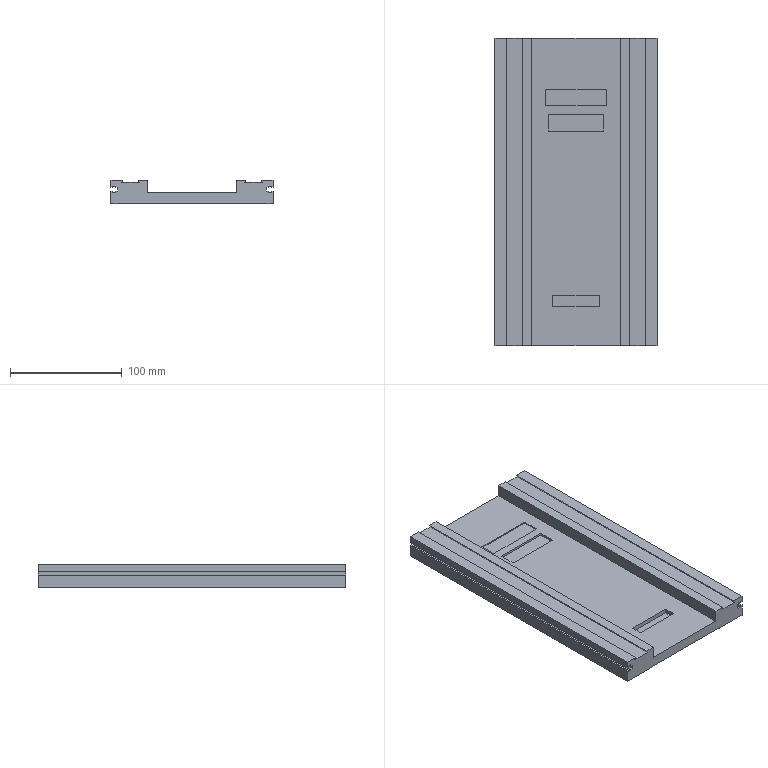Part | NX | features DATUM_CSYS 5, EXTRUDE 5, EXTRACT_BODY 4, SKETCH 4, Container 1, Geometry Instance 1, MOVE_FACE 1, SUBTRACT 1 | 1 solid | 61 faces | box 145 x 275 x 21 mm | volume 550658 mm3 | plane 61